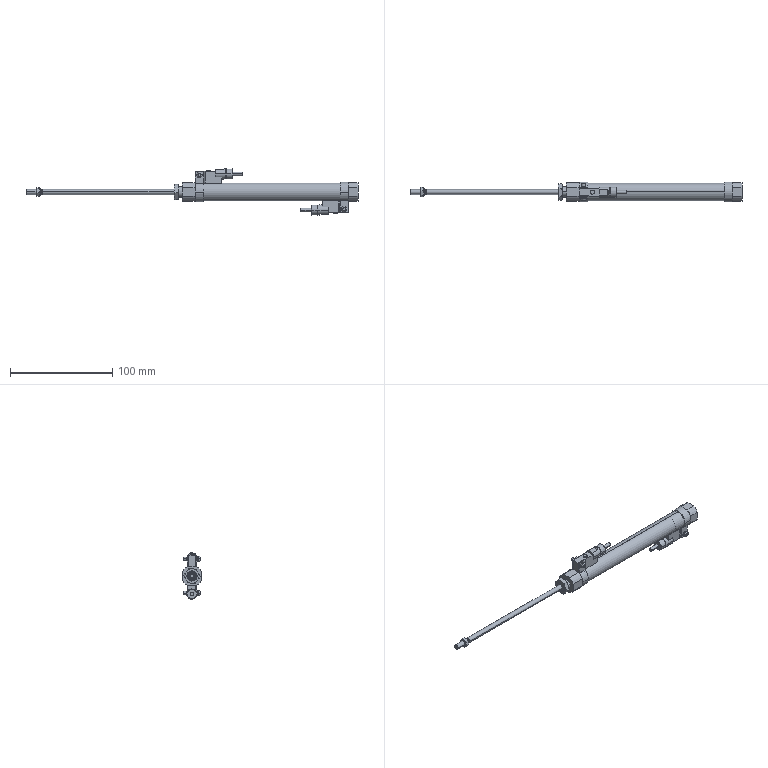Part | SolidWorks | 8 solids | 242 faces | box 325 x 19.2 x 45.4 mm | volume 28867 mm3 | plane 102 | cylinder 92 | cone 44 | torus 4 | commonest cylinder face diameters 3 x16 10 x10 4.134 x8 17.4 x8 17.8 x8 20 x8